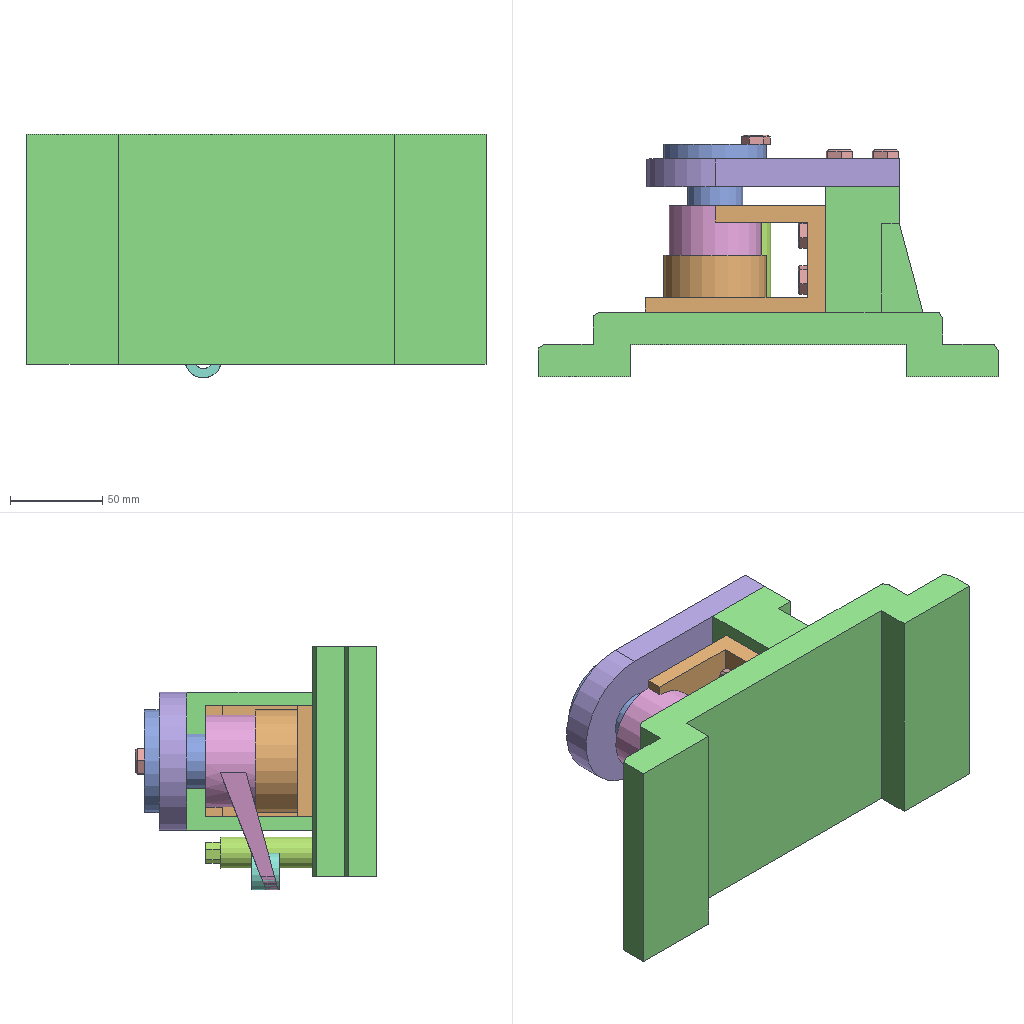Assembly | NX | 7 different items | 15 placed | box 250 x 131 x 133 mm
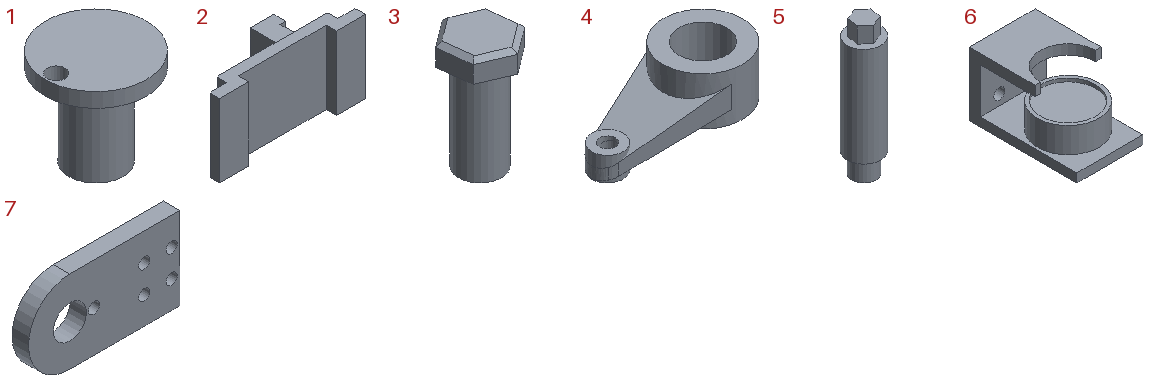Parts list (item | quantity | size | volume | features):
1 | x1 | 56 x 56 x 53 mm | 50884 mm3 | features DATUM_CSYS 4, EXTRUDE 3, SKETCH 3
2 | x1 | 250 x 103.296 x 125 mm | 827680 mm3 | features DATUM_CSYS 8, EXTRUDE 7, SKETCH 6, SIMPLE HOLE 4, DATUM_PLANE 2, OFFSET_REGION 2, CHAMFER 1, CPROJ 1, HOLE PACKAGE 1
3 | x9 | 14.553 x 15.735 x 27 mm | 2520 mm3 | features DATUM_CSYS 3, EXTRUDE 2, SKETCH 2, CHAMFER 1
4 | x1 | 95 x 50 x 40 mm | 53901 mm3 | features DATUM_CSYS 7, EXTRUDE 6, SKETCH 6, REPLACE_FACE 5, DATUM_PLANE 2
5 | x1 | 17 x 17 x 68 mm | 13173 mm3 | features DATUM_CSYS 4, EXTRUDE 3, SKETCH 3, OFFSET_REGION 1
6 | x1 | 60 x 98 x 58 mm | 142821 mm3 | features DATUM_CSYS 12, SKETCH 11, EXTRUDE 6, OFFSET_REGION 4, DATUM_PLANE 2, UNITE 1
7 | x1 | 137.5 x 15 x 75 mm | 129141 mm3 | features DATUM_CSYS 2, EXTRUDE 2, OFFSET_REGION 2, SKETCH 2
Mates (type | each side: item.copy, entity, surface, feature):
Fix | 2.1 component
Touch | 6.1 face plane Extrude(12) | 2.1 face plane Extrude(2)
Concentric | 6.1 edge | 2.1 edge
AlignLock | 4.1 face cylinder Extrude(5) | 6.1 face cylinder Extrude(19)
Concentric | 4.1 edge | 6.1 edge
Concentric | 5.1 edge | 2.1 edge
Concentric | 1.1 edge | 7.1 edge
AlignLock | 1.1 face cylinder Extrude(6) | 7.1 face cylinder Extrude(6)
Concentric | 3.1 edge | 7.1 edge | 4 times
Concentric | 3.1 edge | 1.1 edge
Concentric | 3.1 edge | 6.1 edge | 4 times